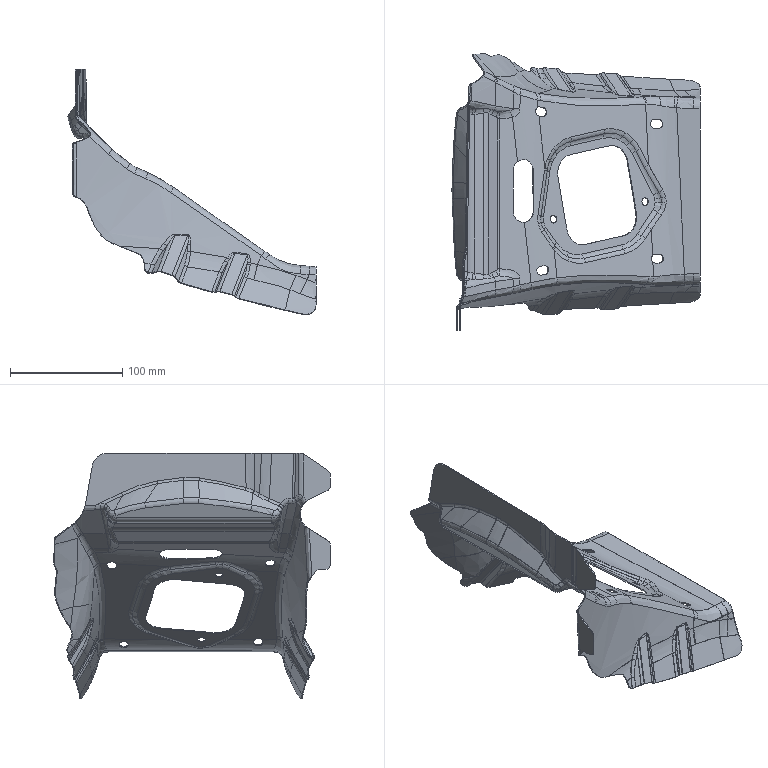Part | 1 solid | 668 faces | box 220.992 x 246.31 x 219.1 mm | volume 76304 mm3 | spline 480 | cylinder 116 | plane 65 | sphere 4 | other 3 | commonest cylinder face diameters 10 x25 12 x23 14 x13 8 x10 34.4 x6 20 x5